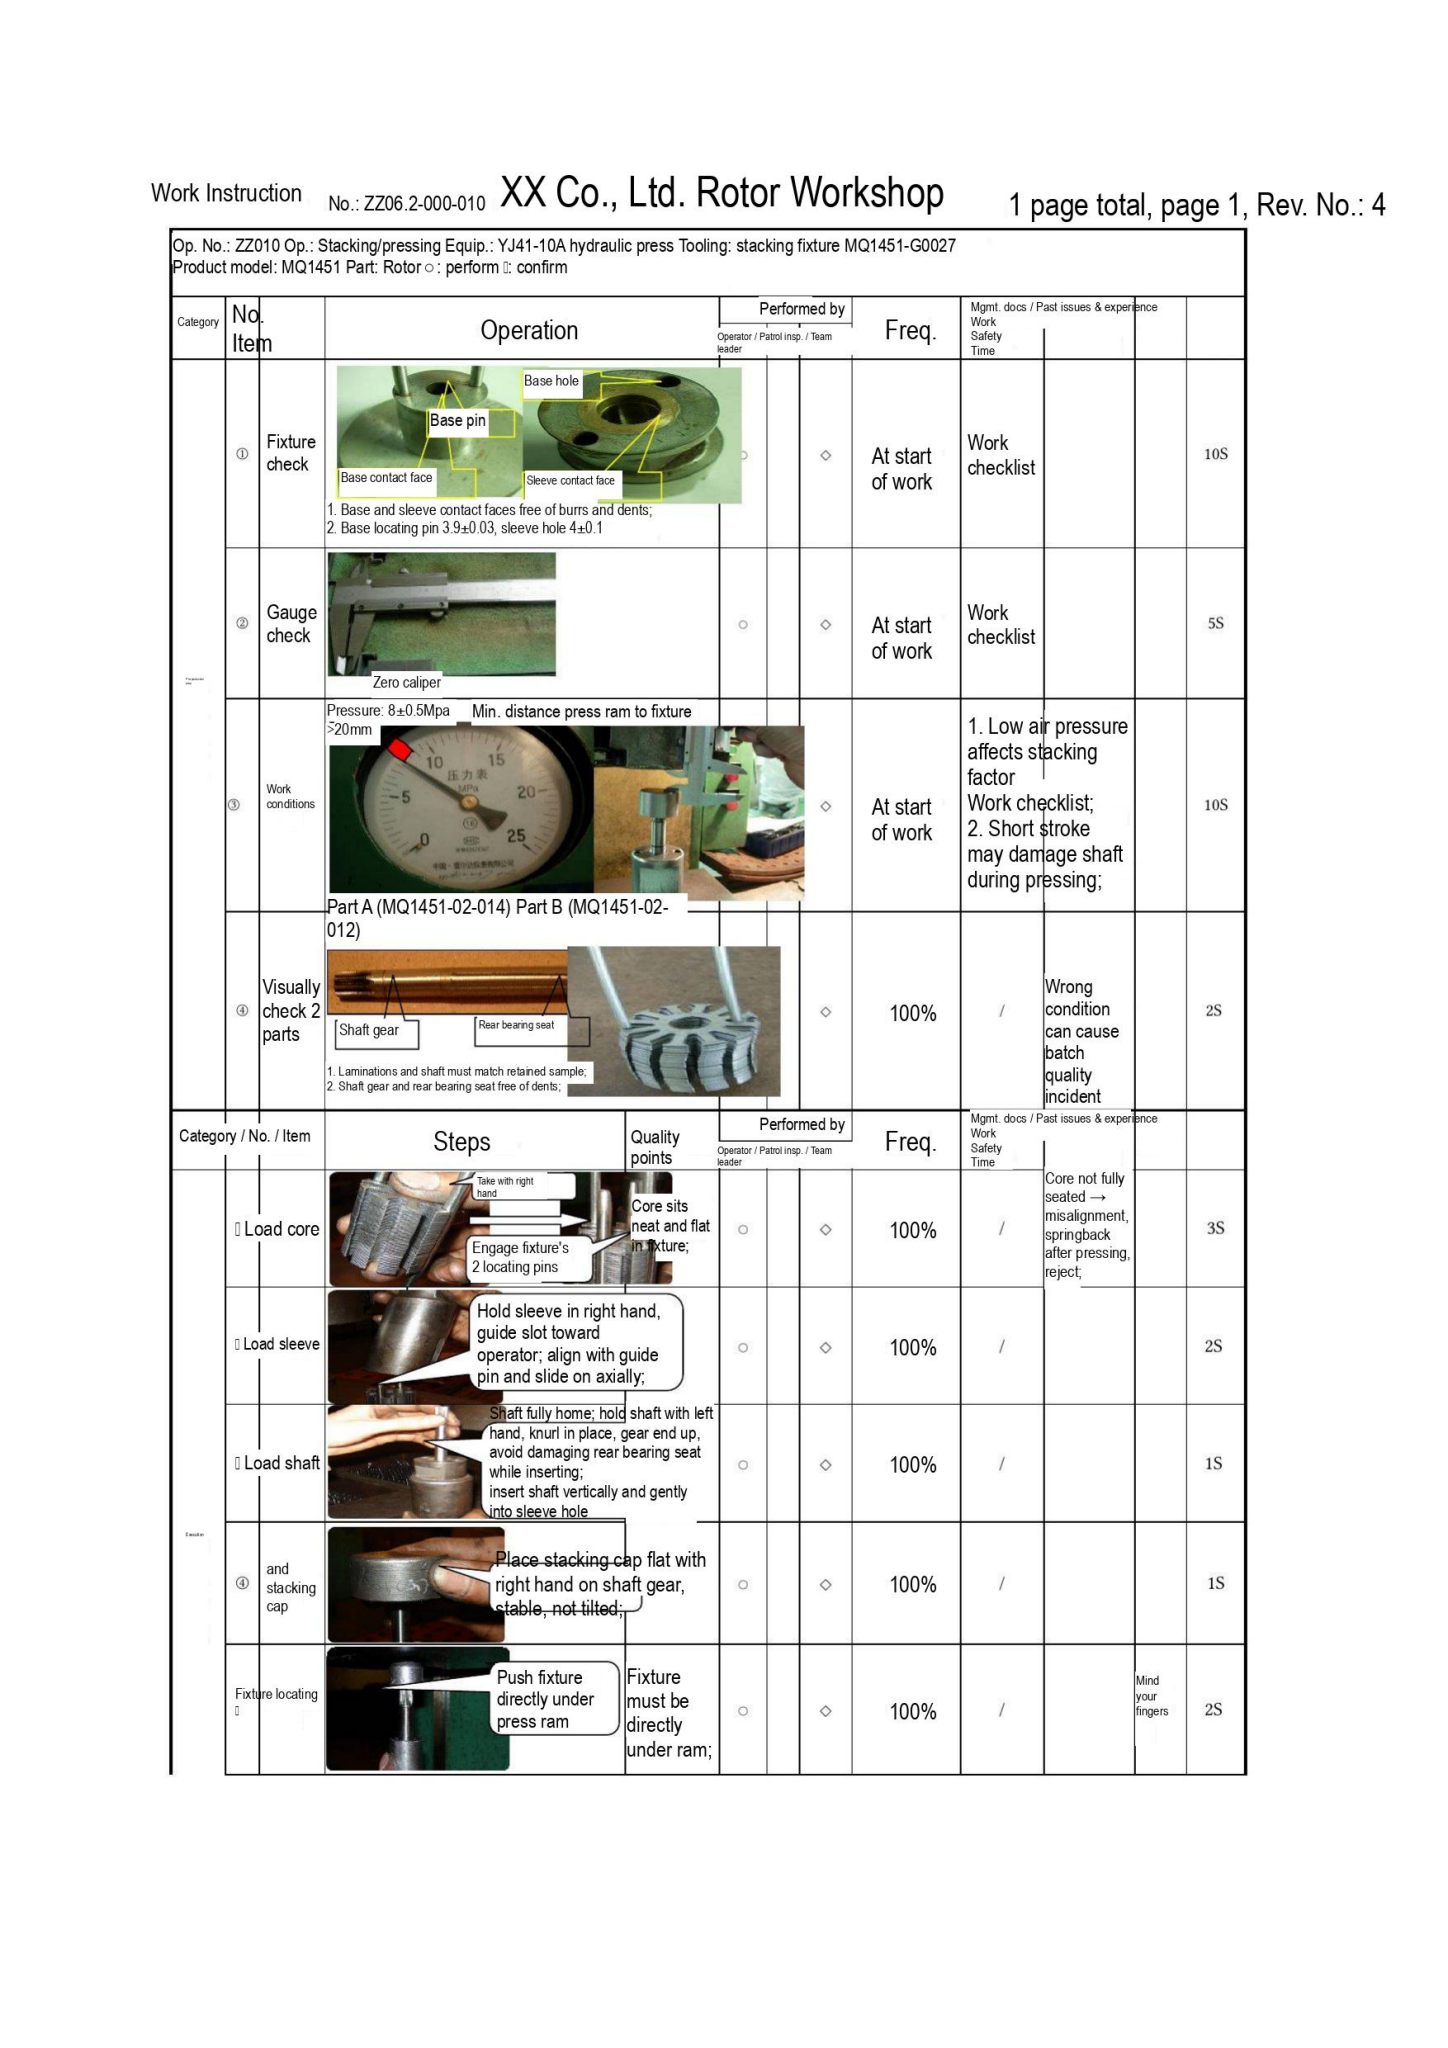Work Instruction No.: ZZ06.2-000-010 XX Co., Ltd. Rotor Workshop 1 page total, page 1, Rev. No.: 4

Op. No.: ZZ010 Op.: Stacking/pressing Equip.: YJ41-10A hydraulic press Tooling: stacking fixture MQ1451-G0027
Product model: MQ1451 Part: Rotor ○: perform ◇: confirm

| Category | No. | Item | Operation | Performed by: Operator | Performed by: Patrol insp. | Performed by: Team leader | Freq. | Mgmt. docs | Past issues & experience: Work | Past issues & experience: Safety | Time |
|---|---|---|---|---|---|---|---|---|---|---|---|
| | ① | Fixture check | Base hole; Base pin; Base contact face; Sleeve contact face<br>1. Base and sleeve contact faces free of burrs and dents;<br>2. Base locating pin 3.9±0.03, sleeve hole 4±0.1 | ○ | ◇ | | At start of work | Work checklist | | | 10S |
| | ② | Gauge check | Zero caliper | ○ | ◇ | | At start of work | Work checklist | | | 5S |
| | ③ | Work conditions | Pressure: 8±0.5Mpa<br>Min. distance press ram to fixture >20mm<br>10 15 压力表 MPa 5 20 0 25 | | ◇ | | At start of work | 1. Low air pressure affects stacking factor<br>Work checklist;<br>2. Short stroke may damage shaft during pressing; | | | 10S |
| | ④ | Visually check 2 parts | Part A (MQ1451-02-014) Part B (MQ1451-02-012)<br>Shaft gear; Rear bearing seat<br>1. Laminations and shaft must match retained sample;<br>2. Shaft gear and rear bearing seat free of dents; | | ◇ | | 100% | / | Wrong condition can cause batch quality incident | | 2S |

| Category / No. / Item | Steps | Quality points | Performed by: Operator | Performed by: Patrol insp. | Performed by: Team leader | Freq. | Mgmt. docs | Past issues & experience: Work | Past issues & experience: Safety | Time |
|---|---|---|---|---|---|---|---|---|---|---|
| Load core | Take with right hand<br>Engage fixture's 2 locating pins | Core sits neat and flat in fixture; | ○ | ◇ | | 100% | / | Core not fully seated → misalignment, springback after pressing, reject; | | 3S |
| Load sleeve | Hold sleeve in right hand, guide slot toward operator; align with guide pin and slide on axially; | | ○ | ◇ | | 100% | / | | | 2S |
| Load shaft | Shaft fully home; hold shaft with left hand, knurl in place, gear end up, avoid damaging rear bearing seat while inserting;<br>insert shaft vertically and gently into sleeve hole | | ○ | ◇ | | 100% | / | | | 1S |
| ④ and stacking cap | Place stacking cap flat with right hand on shaft gear, stable, not tilted; | | ○ | ◇ | | 100% | / | | | 1S |
| Fixture locating | Push fixture directly under press ram | Fixture must be directly under ram; | ○ | ◇ | | 100% | / | | Mind your fingers | 2S |
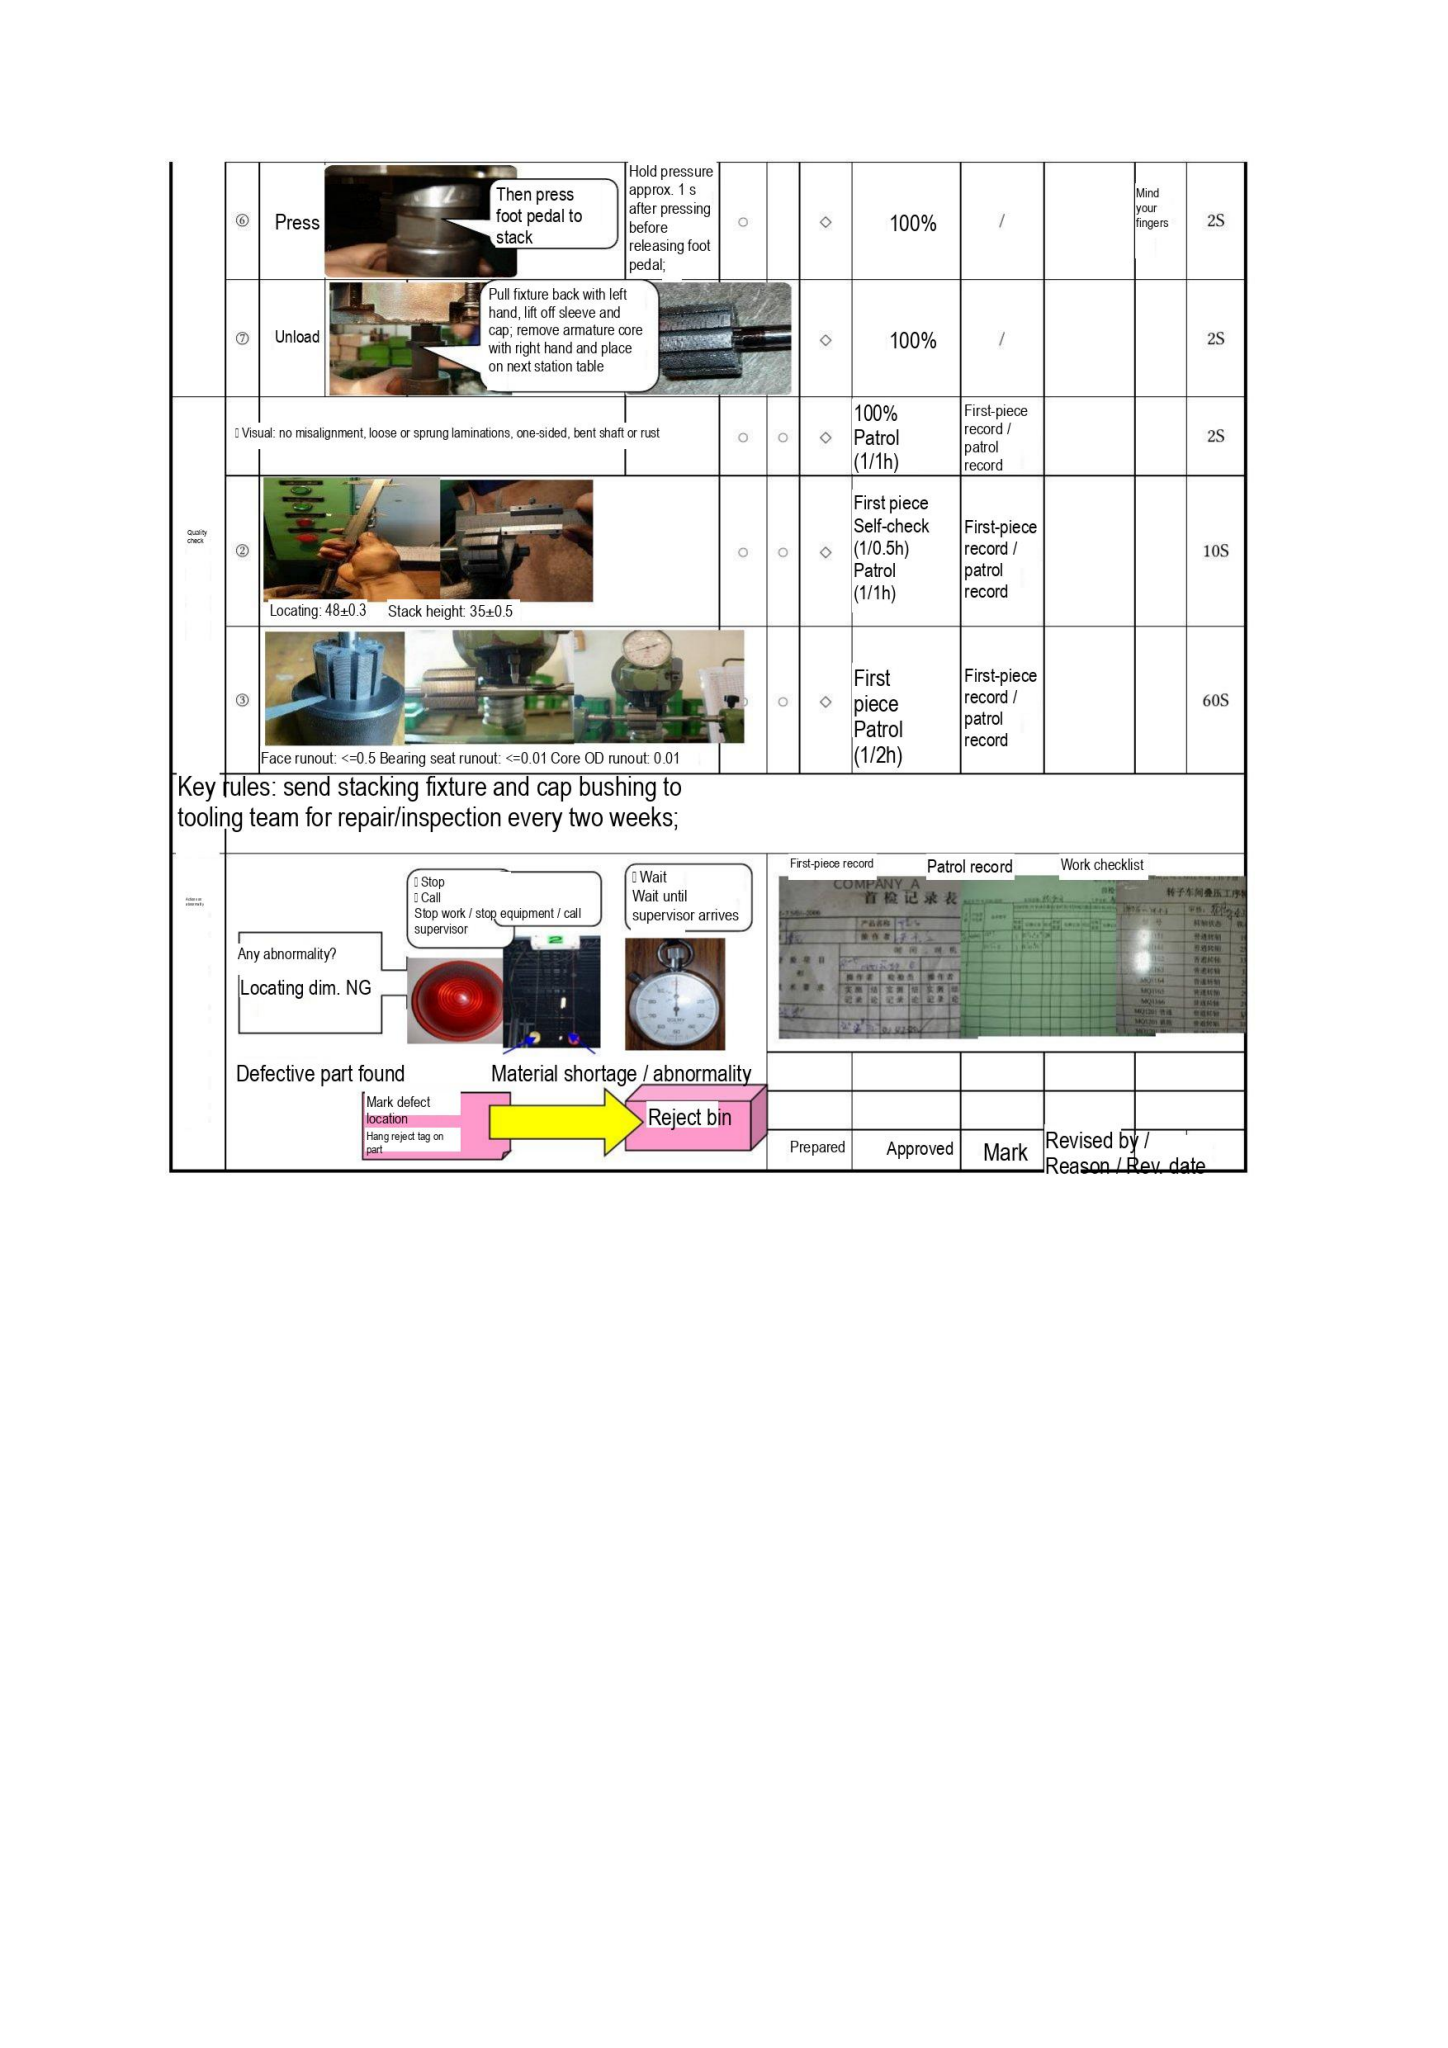| | | | | | | | | | | | | |
|---|---|---|---|---|---|---|---|---|---|---|---|---|
| | ⑥ | Press | Then press foot pedal to stack | Hold pressure approx. 1 s after pressing before releasing foot pedal; | ○ | | ◇ | 100% | / | | Mind your fingers | 2S |
| | ⑦ | Unload | Pull fixture back with left hand, lift off sleeve and cap; remove armature core with right hand and place on next station table | | | | ◇ | 100% | / | | | 2S |
| Quality check | Visual: no misalignment, loose or sprung laminations, one-sided, bent shaft or rust | | | | ○ | ○ | ◇ | 100% Patrol (1/1h) | First-piece record / patrol record | | | 2S |
| | ② | Locating: 48±0.3 Stack height: 35±0.5 | | | ○ | ○ | ◇ | First piece Self-check (1/0.5h) Patrol (1/1h) | First-piece record / patrol record | | | 10S |
| | ③ | Face runout: <=0.5 Bearing seat runout: <=0.01 Core OD runout: 0.01 | | | | ○ | ◇ | First piece Patrol (1/2h) | First-piece record / patrol record | | | 60S |

Key rules: send stacking fixture and cap bushing to tooling team for repair/inspection every two weeks;

Stop
Call
Stop work / stop equipment / call supervisor

Wait
Wait until supervisor arrives

Any abnormality?
Locating dim. NG

Defective part found
Material shortage / abnormality

Mark defect location
Hang reject tag on part

Reject bin

First-piece record
Patrol record
Work checklist

COMPANY A
首 检 记 录 表

| | | | |
|---|---|---|---|
| | | | |
| | | | |
| Prepared | Approved | Mark | Revised by / Reason / Rev. date |